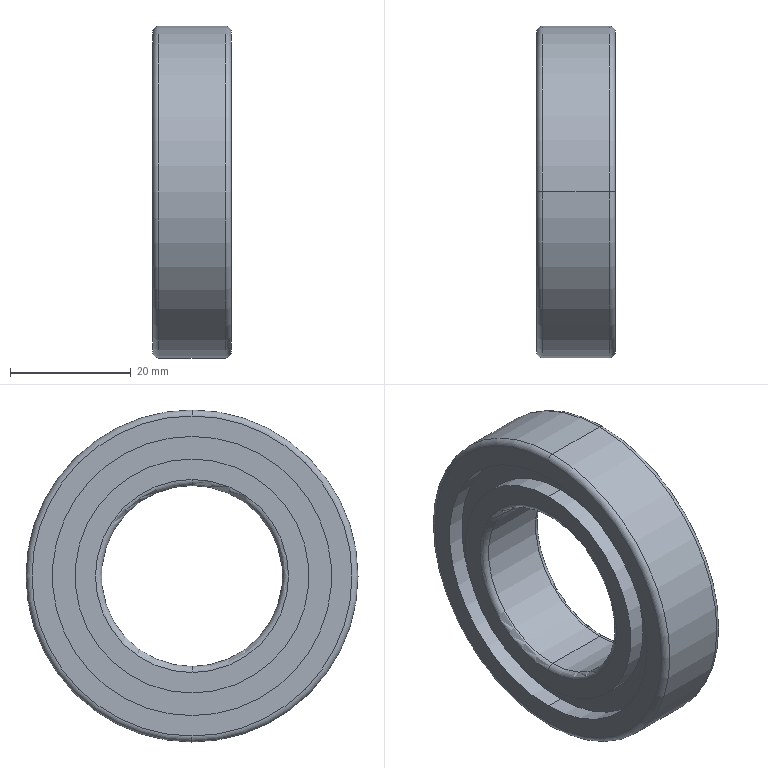Part | STEP file | B6006_B6006 | 1 solid | 26 faces | box 13 x 55 x 55 mm | volume 18718 mm3 | cylinder 12 | torus 8 | plane 6 | commonest cylinder face diameters 38.75 x4 46.25 x4 30 x2 55 x2